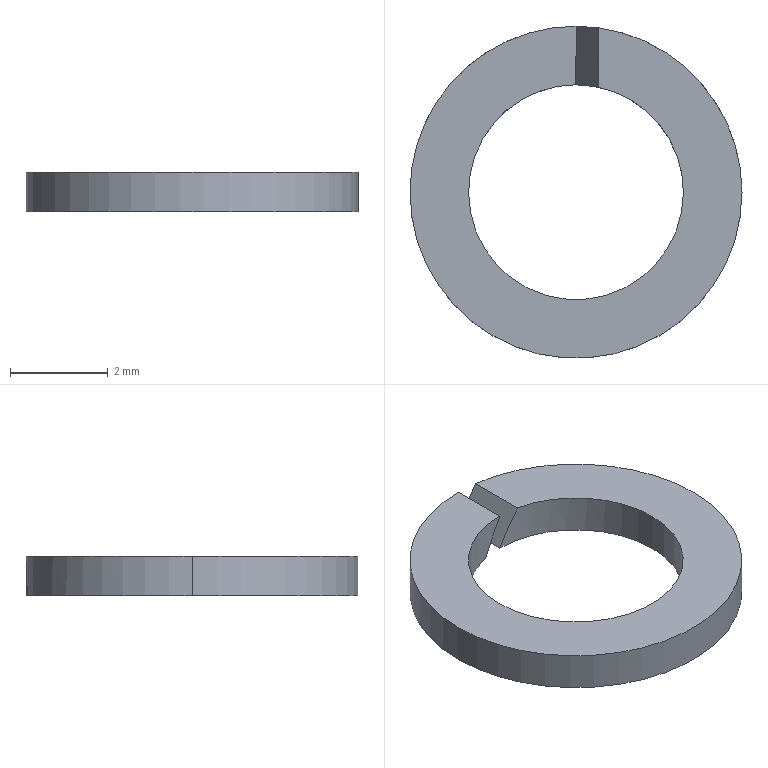Part | NX | features BREP 1 | 1 solid | 10 faces | box 6.8 x 6.8 x 0.8 mm | volume 16.445 mm3 | cylinder 6 | plane 4 | commonest cylinder face diameters 4.4 x3 6.8 x3
STEP:
#1=CARTESIAN_POINT('',(-2.2,0.,-0.8));
#2=VERTEX_POINT('',#1);
#3=CARTESIAN_POINT('',(2.2,0.,-0.8));
#4=VERTEX_POINT('',#3);
#5=CARTESIAN_POINT('',(0.,0.,-0.8));
#6=DIRECTION('',(0.,0.,1.));
#7=DIRECTION('',(1.,0.,0.));
#8=AXIS2_PLACEMENT_3D('',#5,#6,#7);
#9=CIRCLE('',#8,2.2);
#10=EDGE_CURVE('',#2,#4,#9,.T.);
#11=ORIENTED_EDGE('',*,*,#10,.F.);
#12=CARTESIAN_POINT('',(-2.2,0.,0.));
#13=VERTEX_POINT('',#12);
#14=CARTESIAN_POINT('',(-2.2,0.,-0.8));
#15=DIRECTION('',(0.,0.,1.));
#16=VECTOR('',#15,1000.);
#17=LINE('',#14,#16);
#18=EDGE_CURVE('',#2,#13,#17,.T.);
#19=ORIENTED_EDGE('',*,*,#18,.T.);
#20=CARTESIAN_POINT('',(2.2,0.,0.));
#21=VERTEX_POINT('',#20);
#22=CARTESIAN_POINT('',(0.,0.,0.));
#23=DIRECTION('',(0.,0.,1.));
#24=DIRECTION('',(1.,0.,0.));
#25=AXIS2_PLACEMENT_3D('',#22,#23,#24);
#26=CIRCLE('',#25,2.2);
#27=EDGE_CURVE('',#13,#21,#26,.T.);
#28=ORIENTED_EDGE('',*,*,#27,.T.);
#29=CARTESIAN_POINT('',(2.2,0.,-0.8));
#30=DIRECTION('',(0.,0.,1.));
#31=VECTOR('',#30,1000.);
#32=LINE('',#29,#31);
#33=EDGE_CURVE('',#4,#21,#32,.T.);
#34=ORIENTED_EDGE('',*,*,#33,.F.);
#35=EDGE_LOOP('',(#11,#19,#28,#34));
#36=FACE_BOUND('',#35,.T.);
#37=CARTESIAN_POINT('',(0.,0.,-0.8));
#38=DIRECTION('',(0.,0.,1.));
#39=DIRECTION('',(1.,0.,0.));
#40=AXIS2_PLACEMENT_3D('',#37,#38,#39);
#41=CYLINDRICAL_SURFACE('',#40,2.2);
#42=ADVANCED_FACE('',(#36),#41,.F.);
#43=CARTESIAN_POINT('',(-0.4619,3.368,-0.8));
#44=VERTEX_POINT('',#43);
#45=CARTESIAN_POINT('',(-0.4619,2.151,-0.8));
#46=VERTEX_POINT('',#45);
#47=CARTESIAN_POINT('',(-0.4619,2.76,-0.8));
#48=DIRECTION('',(0.,-1.,0.));
#49=VECTOR('',#48,1000.);
#50=LINE('',#47,#49);
#51=EDGE_CURVE('',#44,#46,#50,.T.);
#52=ORIENTED_EDGE('',*,*,#51,.T.);
#53=CARTESIAN_POINT('',(-0.000000002,0.000000002,-0.8));
#54=DIRECTION('',(0.,0.,1.));
#55=DIRECTION('',(1.,0.,0.));
#56=AXIS2_PLACEMENT_3D('',#53,#54,#55);
#57=CIRCLE('',#56,2.2);
#58=EDGE_CURVE('',#46,#2,#57,.T.);
#59=ORIENTED_EDGE('',*,*,#58,.T.);
#60=ORIENTED_EDGE('',*,*,#10,.T.);
#61=CARTESIAN_POINT('',(0.,2.2,-0.8));
#62=VERTEX_POINT('',#61);
#63=CARTESIAN_POINT('',(-0.000000001,-0.000000001,-0.8));
#64=DIRECTION('',(0.,0.,1.));
#65=DIRECTION('',(1.,0.,0.));
#66=AXIS2_PLACEMENT_3D('',#63,#64,#65);
#67=CIRCLE('',#66,2.2);
#68=EDGE_CURVE('',#4,#62,#67,.T.);
#69=ORIENTED_EDGE('',*,*,#68,.T.);
#70=CARTESIAN_POINT('',(0.,3.4,-0.8));
#71=VERTEX_POINT('',#70);
#72=CARTESIAN_POINT('',(0.,2.8,-0.8));
#73=DIRECTION('',(0.,-1.,0.));
#74=VECTOR('',#73,1000.);
#75=LINE('',#72,#74);
#76=EDGE_CURVE('',#71,#62,#75,.T.);
#77=ORIENTED_EDGE('',*,*,#76,.F.);
#78=CARTESIAN_POINT('',(3.4,0.,-0.8));
#79=VERTEX_POINT('',#78);
#80=CARTESIAN_POINT('',(-0.000000004,-0.000000004,-0.8));
#81=DIRECTION('',(0.,0.,1.));
#82=DIRECTION('',(1.,0.,0.));
#83=AXIS2_PLACEMENT_3D('',#80,#81,#82);
#84=CIRCLE('',#83,3.4);
#85=EDGE_CURVE('',#79,#71,#84,.T.);
#86=ORIENTED_EDGE('',*,*,#85,.F.);
#87=CARTESIAN_POINT('',(-3.4,0.,-0.8));
#88=VERTEX_POINT('',#87);
#89=CARTESIAN_POINT('',(0.,0.,-0.8));
#90=DIRECTION('',(0.,0.,1.));
#91=DIRECTION('',(1.,0.,0.));
#92=AXIS2_PLACEMENT_3D('',#89,#90,#91);
#93=CIRCLE('',#92,3.4);
#94=EDGE_CURVE('',#88,#79,#93,.T.);
#95=ORIENTED_EDGE('',*,*,#94,.F.);
#96=CARTESIAN_POINT('',(0.,-0.000000001,-0.8));
#97=DIRECTION('',(0.,0.,1.));
#98=DIRECTION('',(1.,0.,0.));
#99=AXIS2_PLACEMENT_3D('',#96,#97,#98);
#100=CIRCLE('',#99,3.4);
#101=EDGE_CURVE('',#44,#88,#100,.T.);
#102=ORIENTED_EDGE('',*,*,#101,.F.);
#103=EDGE_LOOP('',(#52,#59,#60,#69,#77,#86,#95,#102));
#104=FACE_BOUND('',#103,.T.);
#105=CARTESIAN_POINT('',(0.,0.,-0.8));
#106=DIRECTION('',(0.,0.,1.));
#107=DIRECTION('',(-1.,0.,0.));
#108=AXIS2_PLACEMENT_3D('',#105,#106,#107);
#109=PLANE('',#108);
#110=ADVANCED_FACE('',(#104),#109,.F.);
#111=ORIENTED_EDGE('',*,*,#18,.F.);
#112=ORIENTED_EDGE('',*,*,#58,.F.);
#113=CARTESIAN_POINT('',(0.,2.2,0.));
#114=VERTEX_POINT('',#113);
#115=CARTESIAN_POINT('',(0.,2.2,0.000000001));
#116=CARTESIAN_POINT('',(-0.1545,2.2,-0.2677));
#117=CARTESIAN_POINT('',(-0.3095,2.184,-0.5361));
#118=CARTESIAN_POINT('',(-0.4619,2.151,-0.8));
#119=B_SPLINE_CURVE_WITH_KNOTS('',3,(#115,#116,#117,#118),.UNSPECIFIED.,.F.,.F.,(4,4),(0.,1.),.PIECEWISE_BEZIER_KNOTS.);
#120=EDGE_CURVE('',#114,#46,#119,.T.);
#121=ORIENTED_EDGE('',*,*,#120,.F.);
#122=CARTESIAN_POINT('',(0.,0.,0.000000001));
#123=DIRECTION('',(0.,0.,1.));
#124=DIRECTION('',(1.,0.,0.));
#125=AXIS2_PLACEMENT_3D('',#122,#123,#124);
#126=CIRCLE('',#125,2.2);
#127=EDGE_CURVE('',#114,#13,#126,.T.);
#128=ORIENTED_EDGE('',*,*,#127,.T.);
#129=EDGE_LOOP('',(#111,#112,#121,#128));
#130=FACE_BOUND('',#129,.T.);
#131=CARTESIAN_POINT('',(0.,0.,-0.8));
#132=DIRECTION('',(0.,0.,1.));
#133=DIRECTION('',(-1.,0.,0.));
#134=AXIS2_PLACEMENT_3D('',#131,#132,#133);
#135=CYLINDRICAL_SURFACE('',#134,2.2);
#136=ADVANCED_FACE('',(#130),#135,.F.);
#137=ORIENTED_EDGE('',*,*,#127,.F.);
#138=CARTESIAN_POINT('',(0.,3.4,0.000000001));
#139=VERTEX_POINT('',#138);
#140=CARTESIAN_POINT('',(0.,2.8,0.));
#141=DIRECTION('',(0.,-1.,0.));
#142=VECTOR('',#141,1000.);
#143=LINE('',#140,#142);
#144=EDGE_CURVE('',#139,#114,#143,.T.);
#145=ORIENTED_EDGE('',*,*,#144,.F.);
#146=CARTESIAN_POINT('',(-3.4,0.,0.000000001));
#147=VERTEX_POINT('',#146);
#148=CARTESIAN_POINT('',(0.000000004,-0.000000004,0.));
#149=DIRECTION('',(0.,0.,1.));
#150=DIRECTION('',(1.,0.,0.));
#151=AXIS2_PLACEMENT_3D('',#148,#149,#150);
#152=CIRCLE('',#151,3.4);
#153=EDGE_CURVE('',#139,#147,#152,.T.);
#154=ORIENTED_EDGE('',*,*,#153,.T.);
#155=CARTESIAN_POINT('',(3.4,0.,0.000000001));
#156=VERTEX_POINT('',#155);
#157=CARTESIAN_POINT('',(0.,0.,0.));
#158=DIRECTION('',(0.,0.,1.));
#159=DIRECTION('',(1.,0.,0.));
#160=AXIS2_PLACEMENT_3D('',#157,#158,#159);
#161=CIRCLE('',#160,3.4);
#162=EDGE_CURVE('',#147,#156,#161,.T.);
#163=ORIENTED_EDGE('',*,*,#162,.T.);
#164=CARTESIAN_POINT('',(0.4619,3.368,0.000000001));
#165=VERTEX_POINT('',#164);
#166=CARTESIAN_POINT('',(0.,-0.000000001,0.));
#167=DIRECTION('',(0.,0.,1.));
#168=DIRECTION('',(1.,0.,0.));
#169=AXIS2_PLACEMENT_3D('',#166,#167,#168);
#170=CIRCLE('',#169,3.4);
#171=EDGE_CURVE('',#156,#165,#170,.T.);
#172=ORIENTED_EDGE('',*,*,#171,.T.);
#173=CARTESIAN_POINT('',(0.4619,2.151,0.000000001));
#174=VERTEX_POINT('',#173);
#175=CARTESIAN_POINT('',(0.4619,2.76,0.));
#176=DIRECTION('',(0.,-1.,0.));
#177=VECTOR('',#176,1000.);
#178=LINE('',#175,#177);
#179=EDGE_CURVE('',#165,#174,#178,.T.);
#180=ORIENTED_EDGE('',*,*,#179,.T.);
#181=CARTESIAN_POINT('',(0.000000002,0.000000002,0.));
#182=DIRECTION('',(0.,0.,1.));
#183=DIRECTION('',(1.,0.,0.));
#184=AXIS2_PLACEMENT_3D('',#181,#182,#183);
#185=CIRCLE('',#184,2.2);
#186=EDGE_CURVE('',#21,#174,#185,.T.);
#187=ORIENTED_EDGE('',*,*,#186,.F.);
#188=ORIENTED_EDGE('',*,*,#27,.F.);
#189=EDGE_LOOP('',(#137,#145,#154,#163,#172,#180,#187,#188));
#190=FACE_BOUND('',#189,.T.);
#191=CARTESIAN_POINT('',(0.,0.,0.));
#192=DIRECTION('',(0.,0.,1.));
#193=DIRECTION('',(-1.,0.,0.));
#194=AXIS2_PLACEMENT_3D('',#191,#192,#193);
#195=PLANE('',#194);
#196=ADVANCED_FACE('',(#190),#195,.T.);
#197=ORIENTED_EDGE('',*,*,#68,.F.);
#198=ORIENTED_EDGE('',*,*,#33,.T.);
#199=ORIENTED_EDGE('',*,*,#186,.T.);
#200=CARTESIAN_POINT('',(0.,2.2,-0.8));
#201=CARTESIAN_POINT('',(0.1545,2.2,-0.5323));
#202=CARTESIAN_POINT('',(0.3095,2.184,-0.2639));
#203=CARTESIAN_POINT('',(0.4619,2.151,0.000000001));
#204=B_SPLINE_CURVE_WITH_KNOTS('',3,(#200,#201,#202,#203),.UNSPECIFIED.,.F.,.F.,(4,4),(0.,1.),.PIECEWISE_BEZIER_KNOTS.);
#205=EDGE_CURVE('',#62,#174,#204,.T.);
#206=ORIENTED_EDGE('',*,*,#205,.F.);
#207=EDGE_LOOP('',(#197,#198,#199,#206));
#208=FACE_BOUND('',#207,.T.);
#209=CARTESIAN_POINT('',(0.,0.,-0.8));
#210=DIRECTION('',(0.,0.,1.));
#211=DIRECTION('',(-1.,0.,0.));
#212=AXIS2_PLACEMENT_3D('',#209,#210,#211);
#213=CYLINDRICAL_SURFACE('',#212,2.2);
#214=ADVANCED_FACE('',(#208),#213,.F.);
#215=ORIENTED_EDGE('',*,*,#144,.T.);
#216=ORIENTED_EDGE('',*,*,#120,.T.);
#217=ORIENTED_EDGE('',*,*,#51,.F.);
#218=CARTESIAN_POINT('',(0.,3.4,0.));
#219=CARTESIAN_POINT('',(-0.09251,3.4,-0.1602));
#220=CARTESIAN_POINT('',(-0.1851,3.397,-0.3206));
#221=CARTESIAN_POINT('',(-0.2776,3.391,-0.4808));
#222=CARTESIAN_POINT('',(-0.3699,3.381,-0.6407));
#223=CARTESIAN_POINT('',(-0.4619,3.368,-0.8));
#224=B_SPLINE_CURVE_WITH_KNOTS('',5,(#218,#219,#220,#221,#222,#223),.UNSPECIFIED.,.F.,.F.,(6,6),(0.,1.),.PIECEWISE_BEZIER_KNOTS.);
#225=EDGE_CURVE('',#139,#44,#224,.T.);
#226=ORIENTED_EDGE('',*,*,#225,.F.);
#227=EDGE_LOOP('',(#215,#216,#217,#226));
#228=FACE_BOUND('',#227,.T.);
#229=CARTESIAN_POINT('',(0.,3.4,0.));
#230=DIRECTION('',(0.866,0.,-0.5));
#231=DIRECTION('',(0.5,0.,0.866));
#232=AXIS2_PLACEMENT_3D('',#229,#230,#231);
#233=PLANE('',#232);
#234=ADVANCED_FACE('',(#228),#233,.T.);
#235=ORIENTED_EDGE('',*,*,#76,.T.);
#236=ORIENTED_EDGE('',*,*,#205,.T.);
#237=ORIENTED_EDGE('',*,*,#179,.F.);
#238=CARTESIAN_POINT('',(0.,3.4,-0.8));
#239=CARTESIAN_POINT('',(0.09251,3.4,-0.6398));
#240=CARTESIAN_POINT('',(0.1851,3.397,-0.4794));
#241=CARTESIAN_POINT('',(0.2776,3.391,-0.3192));
#242=CARTESIAN_POINT('',(0.3699,3.381,-0.1593));
#243=CARTESIAN_POINT('',(0.4619,3.368,0.));
#244=B_SPLINE_CURVE_WITH_KNOTS('',5,(#238,#239,#240,#241,#242,#243),.UNSPECIFIED.,.F.,.F.,(6,6),(0.,1.),.PIECEWISE_BEZIER_KNOTS.);
#245=EDGE_CURVE('',#71,#165,#244,.T.);
#246=ORIENTED_EDGE('',*,*,#245,.F.);
#247=EDGE_LOOP('',(#235,#236,#237,#246));
#248=FACE_BOUND('',#247,.T.);
#249=CARTESIAN_POINT('',(0.,3.4,-0.8));
#250=DIRECTION('',(-0.866,0.,0.5));
#251=DIRECTION('',(-0.5,0.,-0.866));
#252=AXIS2_PLACEMENT_3D('',#249,#250,#251);
#253=PLANE('',#252);
#254=ADVANCED_FACE('',(#248),#253,.T.);
#255=CARTESIAN_POINT('',(3.4,0.,-0.8));
#256=DIRECTION('',(0.,0.,1.));
#257=VECTOR('',#256,1000.);
#258=LINE('',#255,#257);
#259=EDGE_CURVE('',#79,#156,#258,.T.);
#260=ORIENTED_EDGE('',*,*,#259,.F.);
#261=ORIENTED_EDGE('',*,*,#85,.T.);
#262=ORIENTED_EDGE('',*,*,#245,.T.);
#263=ORIENTED_EDGE('',*,*,#171,.F.);
#264=EDGE_LOOP('',(#260,#261,#262,#263));
#265=FACE_BOUND('',#264,.T.);
#266=CARTESIAN_POINT('',(0.,0.,-0.8));
#267=DIRECTION('',(0.,0.,1.));
#268=DIRECTION('',(-1.,0.,0.));
#269=AXIS2_PLACEMENT_3D('',#266,#267,#268);
#270=CYLINDRICAL_SURFACE('',#269,3.4);
#271=ADVANCED_FACE('',(#265),#270,.T.);
#272=CARTESIAN_POINT('',(-3.4,0.,-0.8));
#273=DIRECTION('',(0.,0.,1.));
#274=VECTOR('',#273,1000.);
#275=LINE('',#272,#274);
#276=EDGE_CURVE('',#88,#147,#275,.T.);
#277=ORIENTED_EDGE('',*,*,#276,.F.);
#278=ORIENTED_EDGE('',*,*,#94,.T.);
#279=ORIENTED_EDGE('',*,*,#259,.T.);
#280=ORIENTED_EDGE('',*,*,#162,.F.);
#281=EDGE_LOOP('',(#277,#278,#279,#280));
#282=FACE_BOUND('',#281,.T.);
#283=CARTESIAN_POINT('',(0.,0.,-0.8));
#284=DIRECTION('',(0.,0.,1.));
#285=DIRECTION('',(1.,0.,0.));
#286=AXIS2_PLACEMENT_3D('',#283,#284,#285);
#287=CYLINDRICAL_SURFACE('',#286,3.4);
#288=ADVANCED_FACE('',(#282),#287,.T.);
#289=ORIENTED_EDGE('',*,*,#101,.T.);
#290=ORIENTED_EDGE('',*,*,#276,.T.);
#291=ORIENTED_EDGE('',*,*,#153,.F.);
#292=ORIENTED_EDGE('',*,*,#225,.T.);
#293=EDGE_LOOP('',(#289,#290,#291,#292));
#294=FACE_BOUND('',#293,.T.);
#295=CARTESIAN_POINT('',(0.,0.,-0.8));
#296=DIRECTION('',(0.,0.,1.));
#297=DIRECTION('',(-1.,0.,0.));
#298=AXIS2_PLACEMENT_3D('',#295,#296,#297);
#299=CYLINDRICAL_SURFACE('',#298,3.4);
#300=ADVANCED_FACE('',(#294),#299,.T.);
#301=CLOSED_SHELL('',(#42,#110,#136,#196,#214,#234,#254,#271,#288,#300));
#302=MANIFOLD_SOLID_BREP('',#301);
#303=(LENGTH_UNIT()NAMED_UNIT(*)SI_UNIT(.MILLI.,.METRE.));
#304=UNCERTAINTY_MEASURE_WITH_UNIT(LENGTH_MEASURE(0.00001),#303,'','');
#305=(NAMED_UNIT(*)PLANE_ANGLE_UNIT()SI_UNIT($,.RADIAN.));
#306=(NAMED_UNIT(*)SI_UNIT($,.STERADIAN.)SOLID_ANGLE_UNIT());
#307=(GEOMETRIC_REPRESENTATION_CONTEXT(3)GLOBAL_UNCERTAINTY_ASSIGNED_CONTEXT((#304))GLOBAL_UNIT_ASSIGNED_CONTEXT((#303,#305,#306))REPRESENTATION_CONTEXT('',''));
#308=ADVANCED_BREP_SHAPE_REPRESENTATION('',(#302),#307);